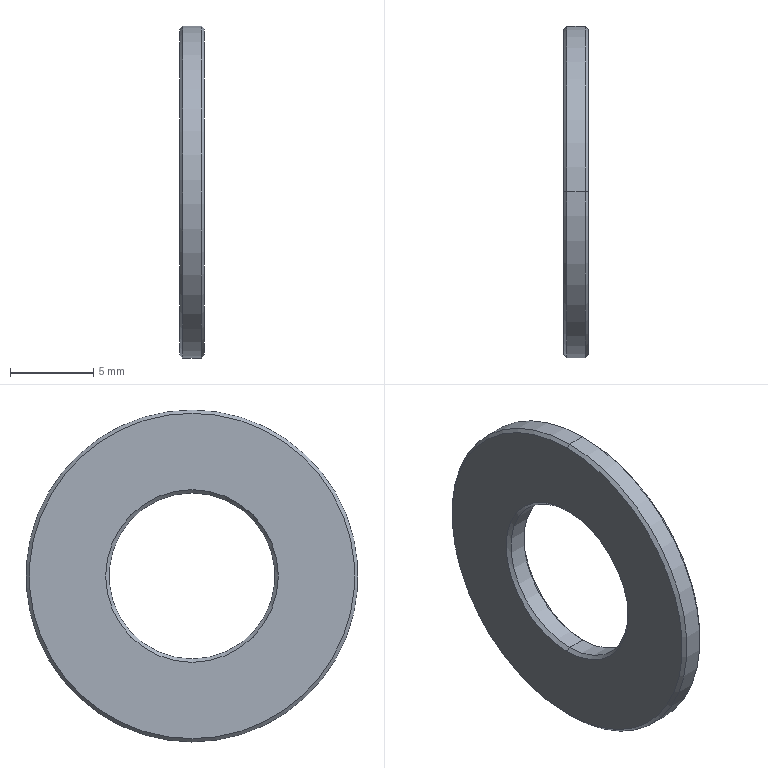Part | STEP file | WSSS20-10-1.5-1 | 1 solid | 14 faces | box 1.5 x 20 x 20 mm | volume 349.659 mm3 | cone 8 | cylinder 4 | plane 2 | commonest cylinder face diameters 10 x2 20 x2
STEP:
#1=CARTESIAN_POINT('',(1.5,0.,-9.8));
#2=VERTEX_POINT('',#1);
#3=CARTESIAN_POINT('',(1.5,0.,9.8));
#4=VERTEX_POINT('',#3);
#5=CARTESIAN_POINT('',(1.5,0.,0.));
#6=DIRECTION('',(1.,0.,0.));
#7=DIRECTION('',(0.,0.,1.));
#8=AXIS2_PLACEMENT_3D('',#5,#6,#7);
#9=CIRCLE('',#8,9.8);
#10=EDGE_CURVE('',#2,#4,#9,.T.);
#11=ORIENTED_EDGE('',*,*,#10,.F.);
#12=CARTESIAN_POINT('',(1.3,0.,-10.));
#13=VERTEX_POINT('',#12);
#14=CARTESIAN_POINT('',(1.3,0.,-10.));
#15=DIRECTION('',(-0.7071,0.,-0.7071));
#16=VECTOR('',#15,1000.);
#17=LINE('',#14,#16);
#18=EDGE_CURVE('',#2,#13,#17,.T.);
#19=ORIENTED_EDGE('',*,*,#18,.T.);
#20=CARTESIAN_POINT('',(1.3,0.,10.));
#21=VERTEX_POINT('',#20);
#22=CARTESIAN_POINT('',(1.3,0.,0.));
#23=DIRECTION('',(-1.,0.,0.));
#24=DIRECTION('',(0.,0.,1.));
#25=AXIS2_PLACEMENT_3D('',#22,#23,#24);
#26=CIRCLE('',#25,10.);
#27=EDGE_CURVE('',#21,#13,#26,.T.);
#28=ORIENTED_EDGE('',*,*,#27,.F.);
#29=CARTESIAN_POINT('',(1.3,0.,10.));
#30=DIRECTION('',(-0.7071,0.,0.7071));
#31=VECTOR('',#30,1000.);
#32=LINE('',#29,#31);
#33=EDGE_CURVE('',#4,#21,#32,.T.);
#34=ORIENTED_EDGE('',*,*,#33,.F.);
#35=EDGE_LOOP('',(#11,#19,#28,#34));
#36=FACE_OUTER_BOUND('',#35,.T.);
#37=CARTESIAN_POINT('',(1.3,0.,0.));
#38=DIRECTION('',(-1.,0.,0.));
#39=DIRECTION('',(0.,0.,1.));
#40=AXIS2_PLACEMENT_3D('',#37,#38,#39);
#41=CONICAL_SURFACE('',#40,10.,0.7854);
#42=ADVANCED_FACE('',(#36),#41,.T.);
#43=CARTESIAN_POINT('',(1.3,0.,5.));
#44=VERTEX_POINT('',#43);
#45=CARTESIAN_POINT('',(1.3,0.,-5.));
#46=VERTEX_POINT('',#45);
#47=CARTESIAN_POINT('',(1.3,0.,0.));
#48=DIRECTION('',(1.,0.,0.));
#49=DIRECTION('',(0.,0.,1.));
#50=AXIS2_PLACEMENT_3D('',#47,#48,#49);
#51=CIRCLE('',#50,5.);
#52=EDGE_CURVE('',#44,#46,#51,.T.);
#53=ORIENTED_EDGE('',*,*,#52,.F.);
#54=CARTESIAN_POINT('',(1.5,0.,5.2));
#55=VERTEX_POINT('',#54);
#56=CARTESIAN_POINT('',(1.5,0.,5.2));
#57=DIRECTION('',(0.7071,0.,0.7071));
#58=VECTOR('',#57,1000.);
#59=LINE('',#56,#58);
#60=EDGE_CURVE('',#44,#55,#59,.T.);
#61=ORIENTED_EDGE('',*,*,#60,.T.);
#62=CARTESIAN_POINT('',(1.5,0.,-5.2));
#63=VERTEX_POINT('',#62);
#64=CARTESIAN_POINT('',(1.5,0.,0.));
#65=DIRECTION('',(-1.,0.,0.));
#66=DIRECTION('',(0.,0.,1.));
#67=AXIS2_PLACEMENT_3D('',#64,#65,#66);
#68=CIRCLE('',#67,5.2);
#69=EDGE_CURVE('',#63,#55,#68,.T.);
#70=ORIENTED_EDGE('',*,*,#69,.F.);
#71=CARTESIAN_POINT('',(1.5,0.,-5.2));
#72=DIRECTION('',(0.7071,0.,-0.7071));
#73=VECTOR('',#72,1000.);
#74=LINE('',#71,#73);
#75=EDGE_CURVE('',#46,#63,#74,.T.);
#76=ORIENTED_EDGE('',*,*,#75,.F.);
#77=EDGE_LOOP('',(#53,#61,#70,#76));
#78=FACE_OUTER_BOUND('',#77,.T.);
#79=CARTESIAN_POINT('',(1.5,0.,0.));
#80=DIRECTION('',(1.,0.,0.));
#81=DIRECTION('',(0.,0.,-1.));
#82=AXIS2_PLACEMENT_3D('',#79,#80,#81);
#83=CONICAL_SURFACE('',#82,5.2,0.7854);
#84=ADVANCED_FACE('',(#78),#83,.F.);
#85=CARTESIAN_POINT('',(0.,0.,9.8));
#86=VERTEX_POINT('',#85);
#87=CARTESIAN_POINT('',(0.,0.,-9.8));
#88=VERTEX_POINT('',#87);
#89=CARTESIAN_POINT('',(0.,0.,0.));
#90=DIRECTION('',(-1.,0.,0.));
#91=DIRECTION('',(0.,0.,-1.));
#92=AXIS2_PLACEMENT_3D('',#89,#90,#91);
#93=CIRCLE('',#92,9.8);
#94=EDGE_CURVE('',#86,#88,#93,.T.);
#95=ORIENTED_EDGE('',*,*,#94,.F.);
#96=CARTESIAN_POINT('',(0.2,0.,10.));
#97=VERTEX_POINT('',#96);
#98=CARTESIAN_POINT('',(0.,0.,9.8));
#99=DIRECTION('',(0.7071,0.,0.7071));
#100=VECTOR('',#99,1000.);
#101=LINE('',#98,#100);
#102=EDGE_CURVE('',#86,#97,#101,.T.);
#103=ORIENTED_EDGE('',*,*,#102,.T.);
#104=CARTESIAN_POINT('',(0.2,0.,-10.));
#105=VERTEX_POINT('',#104);
#106=CARTESIAN_POINT('',(0.2,0.,0.));
#107=DIRECTION('',(1.,0.,0.));
#108=DIRECTION('',(0.,0.,-1.));
#109=AXIS2_PLACEMENT_3D('',#106,#107,#108);
#110=CIRCLE('',#109,10.);
#111=EDGE_CURVE('',#105,#97,#110,.T.);
#112=ORIENTED_EDGE('',*,*,#111,.F.);
#113=CARTESIAN_POINT('',(0.,0.,-9.8));
#114=DIRECTION('',(0.7071,0.,-0.7071));
#115=VECTOR('',#114,1000.);
#116=LINE('',#113,#115);
#117=EDGE_CURVE('',#88,#105,#116,.T.);
#118=ORIENTED_EDGE('',*,*,#117,.F.);
#119=EDGE_LOOP('',(#95,#103,#112,#118));
#120=FACE_OUTER_BOUND('',#119,.T.);
#121=CARTESIAN_POINT('',(0.,0.,0.));
#122=DIRECTION('',(1.,0.,0.));
#123=DIRECTION('',(0.,0.,-1.));
#124=AXIS2_PLACEMENT_3D('',#121,#122,#123);
#125=CONICAL_SURFACE('',#124,9.8,0.7854);
#126=ADVANCED_FACE('',(#120),#125,.T.);
#127=CARTESIAN_POINT('',(0.2,0.,-5.));
#128=VERTEX_POINT('',#127);
#129=CARTESIAN_POINT('',(0.2,0.,5.));
#130=VERTEX_POINT('',#129);
#131=CARTESIAN_POINT('',(0.2,0.,0.));
#132=DIRECTION('',(-1.,0.,0.));
#133=DIRECTION('',(0.,0.,-1.));
#134=AXIS2_PLACEMENT_3D('',#131,#132,#133);
#135=CIRCLE('',#134,5.);
#136=EDGE_CURVE('',#128,#130,#135,.T.);
#137=ORIENTED_EDGE('',*,*,#136,.F.);
#138=CARTESIAN_POINT('',(0.,0.,-5.2));
#139=VERTEX_POINT('',#138);
#140=CARTESIAN_POINT('',(0.2,0.,-5.));
#141=DIRECTION('',(-0.7071,0.,-0.7071));
#142=VECTOR('',#141,1000.);
#143=LINE('',#140,#142);
#144=EDGE_CURVE('',#128,#139,#143,.T.);
#145=ORIENTED_EDGE('',*,*,#144,.T.);
#146=CARTESIAN_POINT('',(0.,0.,5.2));
#147=VERTEX_POINT('',#146);
#148=CARTESIAN_POINT('',(0.,0.,0.));
#149=DIRECTION('',(1.,0.,0.));
#150=DIRECTION('',(0.,0.,-1.));
#151=AXIS2_PLACEMENT_3D('',#148,#149,#150);
#152=CIRCLE('',#151,5.2);
#153=EDGE_CURVE('',#147,#139,#152,.T.);
#154=ORIENTED_EDGE('',*,*,#153,.F.);
#155=CARTESIAN_POINT('',(0.2,0.,5.));
#156=DIRECTION('',(-0.7071,0.,0.7071));
#157=VECTOR('',#156,1000.);
#158=LINE('',#155,#157);
#159=EDGE_CURVE('',#130,#147,#158,.T.);
#160=ORIENTED_EDGE('',*,*,#159,.F.);
#161=EDGE_LOOP('',(#137,#145,#154,#160));
#162=FACE_OUTER_BOUND('',#161,.T.);
#163=CARTESIAN_POINT('',(0.2,0.,0.));
#164=DIRECTION('',(-1.,0.,0.));
#165=DIRECTION('',(0.,0.,1.));
#166=AXIS2_PLACEMENT_3D('',#163,#164,#165);
#167=CONICAL_SURFACE('',#166,5.,0.7854);
#168=ADVANCED_FACE('',(#162),#167,.F.);
#169=ORIENTED_EDGE('',*,*,#52,.T.);
#170=CARTESIAN_POINT('',(0.,0.,-5.));
#171=DIRECTION('',(-1.,0.,0.));
#172=VECTOR('',#171,1000.);
#173=LINE('',#170,#172);
#174=EDGE_CURVE('',#46,#128,#173,.T.);
#175=ORIENTED_EDGE('',*,*,#174,.T.);
#176=ORIENTED_EDGE('',*,*,#136,.T.);
#177=CARTESIAN_POINT('',(0.,0.,5.));
#178=DIRECTION('',(-1.,0.,0.));
#179=VECTOR('',#178,1000.);
#180=LINE('',#177,#179);
#181=EDGE_CURVE('',#44,#130,#180,.T.);
#182=ORIENTED_EDGE('',*,*,#181,.F.);
#183=EDGE_LOOP('',(#169,#175,#176,#182));
#184=FACE_OUTER_BOUND('',#183,.T.);
#185=CARTESIAN_POINT('',(0.,0.,0.));
#186=DIRECTION('',(-1.,0.,0.));
#187=DIRECTION('',(0.,0.,1.));
#188=AXIS2_PLACEMENT_3D('',#185,#186,#187);
#189=CYLINDRICAL_SURFACE('',#188,5.);
#190=ADVANCED_FACE('',(#184),#189,.F.);
#191=ORIENTED_EDGE('',*,*,#27,.T.);
#192=CARTESIAN_POINT('',(0.,0.,-10.));
#193=DIRECTION('',(-1.,0.,0.));
#194=VECTOR('',#193,1000.);
#195=LINE('',#192,#194);
#196=EDGE_CURVE('',#13,#105,#195,.T.);
#197=ORIENTED_EDGE('',*,*,#196,.T.);
#198=ORIENTED_EDGE('',*,*,#111,.T.);
#199=CARTESIAN_POINT('',(0.,0.,10.));
#200=DIRECTION('',(-1.,0.,0.));
#201=VECTOR('',#200,1000.);
#202=LINE('',#199,#201);
#203=EDGE_CURVE('',#21,#97,#202,.T.);
#204=ORIENTED_EDGE('',*,*,#203,.F.);
#205=EDGE_LOOP('',(#191,#197,#198,#204));
#206=FACE_OUTER_BOUND('',#205,.T.);
#207=CARTESIAN_POINT('',(0.,0.,0.));
#208=DIRECTION('',(-1.,0.,0.));
#209=DIRECTION('',(0.,0.,1.));
#210=AXIS2_PLACEMENT_3D('',#207,#208,#209);
#211=CYLINDRICAL_SURFACE('',#210,10.);
#212=ADVANCED_FACE('',(#206),#211,.T.);
#213=ORIENTED_EDGE('',*,*,#153,.T.);
#214=CARTESIAN_POINT('',(0.,0.,0.));
#215=DIRECTION('',(1.,0.,0.));
#216=DIRECTION('',(0.,0.,-1.));
#217=AXIS2_PLACEMENT_3D('',#214,#215,#216);
#218=CIRCLE('',#217,5.2);
#219=EDGE_CURVE('',#139,#147,#218,.T.);
#220=ORIENTED_EDGE('',*,*,#219,.T.);
#221=EDGE_LOOP('',(#213,#220));
#222=FACE_BOUND('',#221,.T.);
#223=CARTESIAN_POINT('',(0.,0.,0.));
#224=DIRECTION('',(-1.,0.,0.));
#225=DIRECTION('',(0.,0.,-1.));
#226=AXIS2_PLACEMENT_3D('',#223,#224,#225);
#227=CIRCLE('',#226,9.8);
#228=EDGE_CURVE('',#88,#86,#227,.T.);
#229=ORIENTED_EDGE('',*,*,#228,.T.);
#230=ORIENTED_EDGE('',*,*,#94,.T.);
#231=EDGE_LOOP('',(#229,#230));
#232=FACE_OUTER_BOUND('',#231,.T.);
#233=CARTESIAN_POINT('',(0.,5.,0.));
#234=DIRECTION('',(1.,0.,0.));
#235=DIRECTION('',(0.,0.,-1.));
#236=AXIS2_PLACEMENT_3D('',#233,#234,#235);
#237=PLANE('',#236);
#238=ADVANCED_FACE('',(#222,#232),#237,.F.);
#239=ORIENTED_EDGE('',*,*,#196,.F.);
#240=CARTESIAN_POINT('',(1.3,0.,0.));
#241=DIRECTION('',(-1.,0.,0.));
#242=DIRECTION('',(0.,0.,1.));
#243=AXIS2_PLACEMENT_3D('',#240,#241,#242);
#244=CIRCLE('',#243,10.);
#245=EDGE_CURVE('',#13,#21,#244,.T.);
#246=ORIENTED_EDGE('',*,*,#245,.T.);
#247=ORIENTED_EDGE('',*,*,#203,.T.);
#248=CARTESIAN_POINT('',(0.2,0.,0.));
#249=DIRECTION('',(1.,0.,0.));
#250=DIRECTION('',(0.,0.,-1.));
#251=AXIS2_PLACEMENT_3D('',#248,#249,#250);
#252=CIRCLE('',#251,10.);
#253=EDGE_CURVE('',#97,#105,#252,.T.);
#254=ORIENTED_EDGE('',*,*,#253,.T.);
#255=EDGE_LOOP('',(#239,#246,#247,#254));
#256=FACE_OUTER_BOUND('',#255,.T.);
#257=CARTESIAN_POINT('',(0.,0.,0.));
#258=DIRECTION('',(-1.,0.,0.));
#259=DIRECTION('',(0.,0.,1.));
#260=AXIS2_PLACEMENT_3D('',#257,#258,#259);
#261=CYLINDRICAL_SURFACE('',#260,10.);
#262=ADVANCED_FACE('',(#256),#261,.T.);
#263=ORIENTED_EDGE('',*,*,#69,.T.);
#264=CARTESIAN_POINT('',(1.5,0.,0.));
#265=DIRECTION('',(-1.,0.,0.));
#266=DIRECTION('',(0.,0.,1.));
#267=AXIS2_PLACEMENT_3D('',#264,#265,#266);
#268=CIRCLE('',#267,5.2);
#269=EDGE_CURVE('',#55,#63,#268,.T.);
#270=ORIENTED_EDGE('',*,*,#269,.T.);
#271=EDGE_LOOP('',(#263,#270));
#272=FACE_BOUND('',#271,.T.);
#273=CARTESIAN_POINT('',(1.5,0.,0.));
#274=DIRECTION('',(1.,0.,0.));
#275=DIRECTION('',(0.,0.,1.));
#276=AXIS2_PLACEMENT_3D('',#273,#274,#275);
#277=CIRCLE('',#276,9.8);
#278=EDGE_CURVE('',#4,#2,#277,.T.);
#279=ORIENTED_EDGE('',*,*,#278,.T.);
#280=ORIENTED_EDGE('',*,*,#10,.T.);
#281=EDGE_LOOP('',(#279,#280));
#282=FACE_OUTER_BOUND('',#281,.T.);
#283=CARTESIAN_POINT('',(1.5,5.,0.));
#284=DIRECTION('',(-1.,0.,0.));
#285=DIRECTION('',(0.,0.,1.));
#286=AXIS2_PLACEMENT_3D('',#283,#284,#285);
#287=PLANE('',#286);
#288=ADVANCED_FACE('',(#272,#282),#287,.F.);
#289=ORIENTED_EDGE('',*,*,#174,.F.);
#290=CARTESIAN_POINT('',(1.3,0.,0.));
#291=DIRECTION('',(1.,0.,0.));
#292=DIRECTION('',(0.,0.,1.));
#293=AXIS2_PLACEMENT_3D('',#290,#291,#292);
#294=CIRCLE('',#293,5.);
#295=EDGE_CURVE('',#46,#44,#294,.T.);
#296=ORIENTED_EDGE('',*,*,#295,.T.);
#297=ORIENTED_EDGE('',*,*,#181,.T.);
#298=CARTESIAN_POINT('',(0.2,0.,0.));
#299=DIRECTION('',(-1.,0.,0.));
#300=DIRECTION('',(0.,0.,-1.));
#301=AXIS2_PLACEMENT_3D('',#298,#299,#300);
#302=CIRCLE('',#301,5.);
#303=EDGE_CURVE('',#130,#128,#302,.T.);
#304=ORIENTED_EDGE('',*,*,#303,.T.);
#305=EDGE_LOOP('',(#289,#296,#297,#304));
#306=FACE_OUTER_BOUND('',#305,.T.);
#307=CARTESIAN_POINT('',(0.,0.,0.));
#308=DIRECTION('',(-1.,0.,0.));
#309=DIRECTION('',(0.,0.,1.));
#310=AXIS2_PLACEMENT_3D('',#307,#308,#309);
#311=CYLINDRICAL_SURFACE('',#310,5.);
#312=ADVANCED_FACE('',(#306),#311,.F.);
#313=ORIENTED_EDGE('',*,*,#144,.F.);
#314=ORIENTED_EDGE('',*,*,#303,.F.);
#315=ORIENTED_EDGE('',*,*,#159,.T.);
#316=ORIENTED_EDGE('',*,*,#219,.F.);
#317=EDGE_LOOP('',(#313,#314,#315,#316));
#318=FACE_OUTER_BOUND('',#317,.T.);
#319=CARTESIAN_POINT('',(0.2,0.,0.));
#320=DIRECTION('',(-1.,0.,0.));
#321=DIRECTION('',(0.,0.,1.));
#322=AXIS2_PLACEMENT_3D('',#319,#320,#321);
#323=CONICAL_SURFACE('',#322,5.,0.7854);
#324=ADVANCED_FACE('',(#318),#323,.F.);
#325=ORIENTED_EDGE('',*,*,#102,.F.);
#326=ORIENTED_EDGE('',*,*,#228,.F.);
#327=ORIENTED_EDGE('',*,*,#117,.T.);
#328=ORIENTED_EDGE('',*,*,#253,.F.);
#329=EDGE_LOOP('',(#325,#326,#327,#328));
#330=FACE_OUTER_BOUND('',#329,.T.);
#331=CARTESIAN_POINT('',(0.,0.,0.));
#332=DIRECTION('',(1.,0.,0.));
#333=DIRECTION('',(0.,0.,-1.));
#334=AXIS2_PLACEMENT_3D('',#331,#332,#333);
#335=CONICAL_SURFACE('',#334,9.8,0.7854);
#336=ADVANCED_FACE('',(#330),#335,.T.);
#337=ORIENTED_EDGE('',*,*,#60,.F.);
#338=ORIENTED_EDGE('',*,*,#295,.F.);
#339=ORIENTED_EDGE('',*,*,#75,.T.);
#340=ORIENTED_EDGE('',*,*,#269,.F.);
#341=EDGE_LOOP('',(#337,#338,#339,#340));
#342=FACE_OUTER_BOUND('',#341,.T.);
#343=CARTESIAN_POINT('',(1.5,0.,0.));
#344=DIRECTION('',(1.,0.,0.));
#345=DIRECTION('',(0.,0.,-1.));
#346=AXIS2_PLACEMENT_3D('',#343,#344,#345);
#347=CONICAL_SURFACE('',#346,5.2,0.7854);
#348=ADVANCED_FACE('',(#342),#347,.F.);
#349=ORIENTED_EDGE('',*,*,#18,.F.);
#350=ORIENTED_EDGE('',*,*,#278,.F.);
#351=ORIENTED_EDGE('',*,*,#33,.T.);
#352=ORIENTED_EDGE('',*,*,#245,.F.);
#353=EDGE_LOOP('',(#349,#350,#351,#352));
#354=FACE_OUTER_BOUND('',#353,.T.);
#355=CARTESIAN_POINT('',(1.3,0.,0.));
#356=DIRECTION('',(-1.,0.,0.));
#357=DIRECTION('',(0.,0.,1.));
#358=AXIS2_PLACEMENT_3D('',#355,#356,#357);
#359=CONICAL_SURFACE('',#358,10.,0.7854);
#360=ADVANCED_FACE('',(#354),#359,.T.);
#361=CLOSED_SHELL('',(#42,#84,#126,#168,#190,#212,#238,#262,#288,#312,#324,#336,#348,#360));
#362=MANIFOLD_SOLID_BREP('',#361);
#363=CARTESIAN_POINT('',(0.,0.,0.));
#364=DIRECTION('',(0.,0.,1.));
#365=DIRECTION('',(1.,0.,0.));
#366=AXIS2_PLACEMENT_3D('',#363,#364,#365);
#367=(LENGTH_UNIT()NAMED_UNIT(*)SI_UNIT(.MILLI.,.METRE.));
#368=UNCERTAINTY_MEASURE_WITH_UNIT(LENGTH_MEASURE(0.00001),#367,'','');
#369=(NAMED_UNIT(*)PLANE_ANGLE_UNIT()SI_UNIT($,.RADIAN.));
#370=(NAMED_UNIT(*)SI_UNIT($,.STERADIAN.)SOLID_ANGLE_UNIT());
#371=(GEOMETRIC_REPRESENTATION_CONTEXT(3)GLOBAL_UNCERTAINTY_ASSIGNED_CONTEXT((#368))GLOBAL_UNIT_ASSIGNED_CONTEXT((#367,#369,#370))REPRESENTATION_CONTEXT('',''));
#372=ADVANCED_BREP_SHAPE_REPRESENTATION('',(#362,#366),#371);